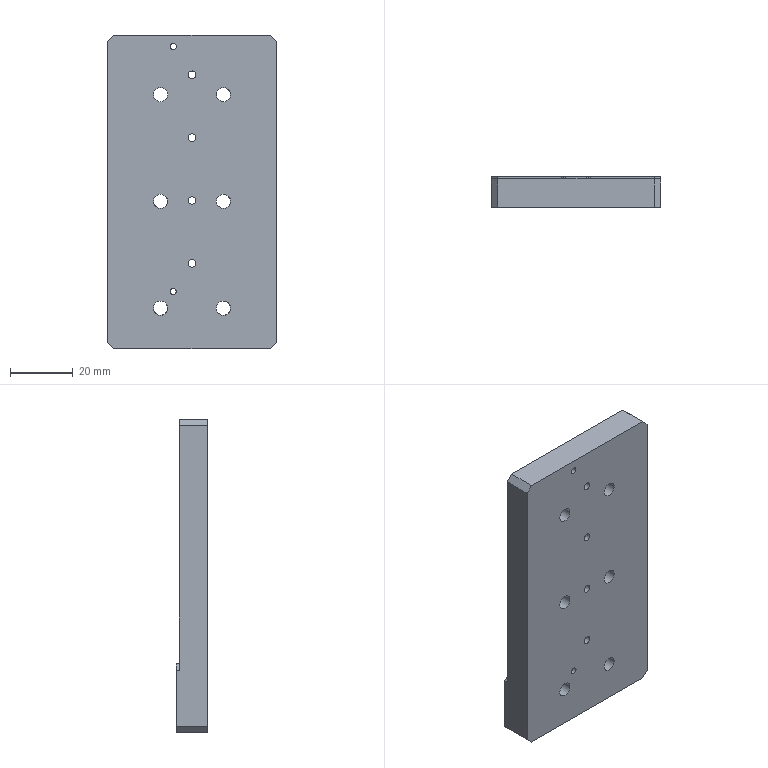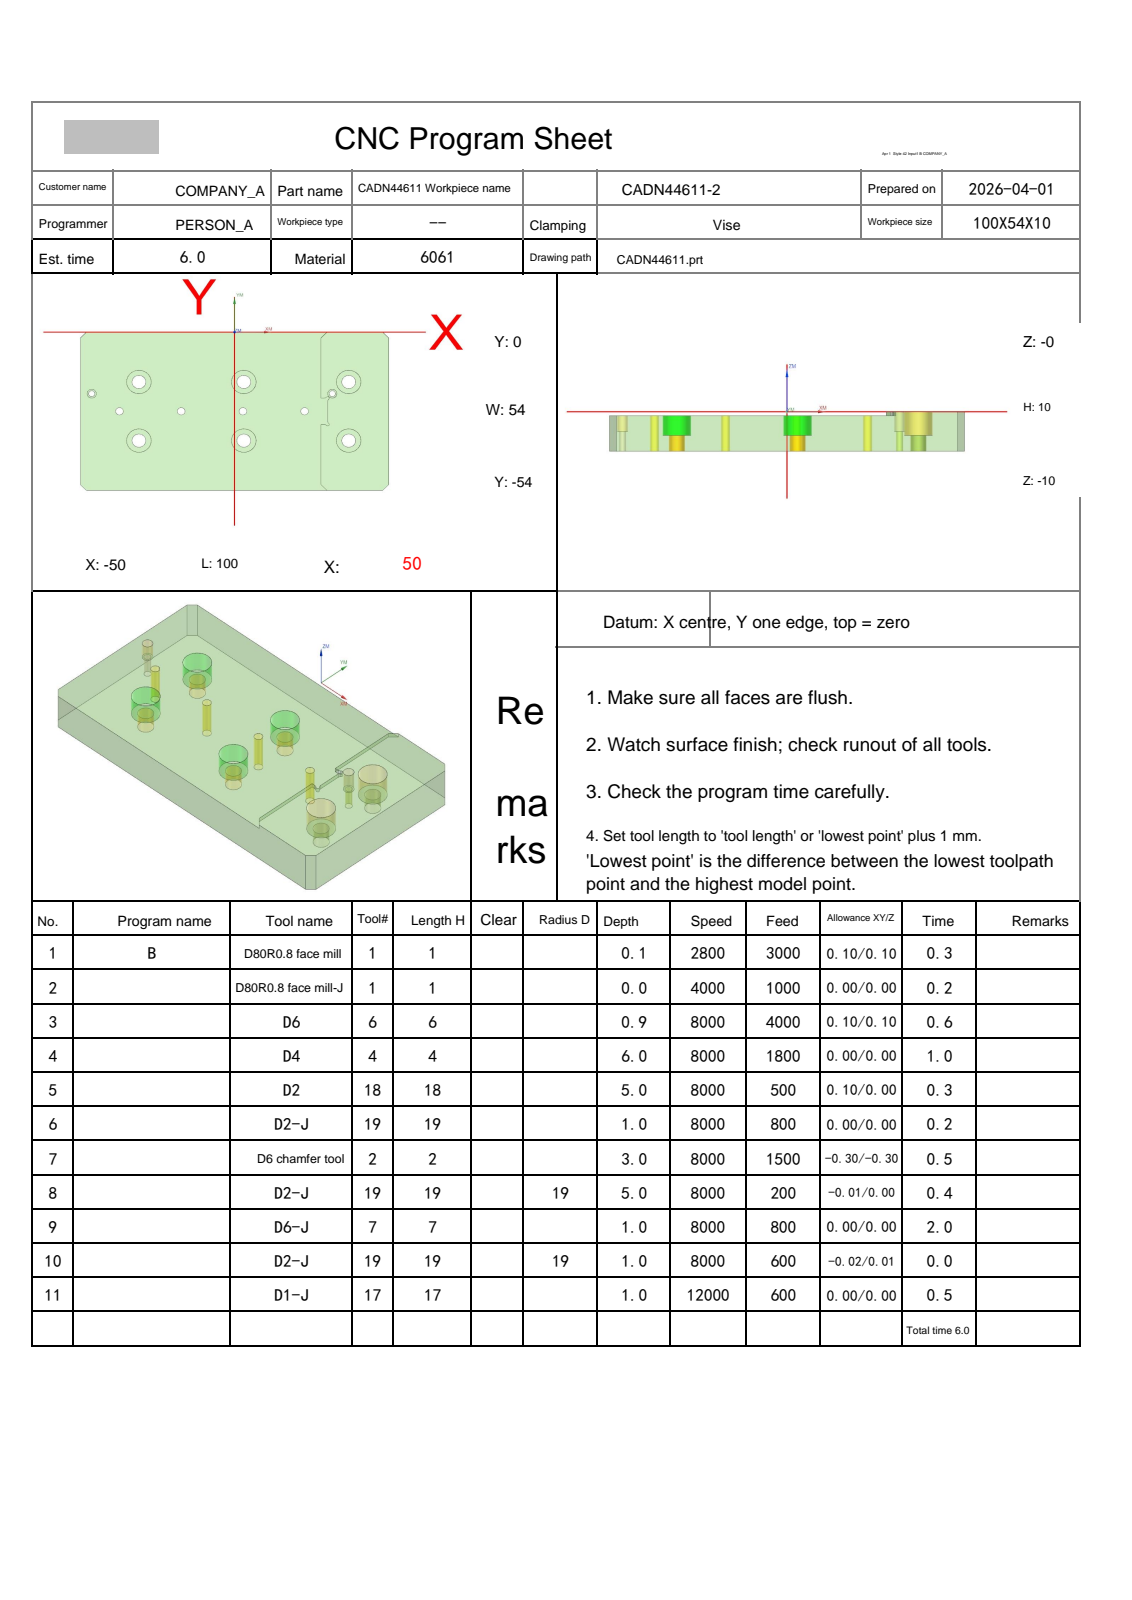NC program | NX | posted by the shop | part box 54 x 10 x 100 mm
Lines 1971 to 3760 of 3760, first 1687 of 1790 lines:
N11 T17 M06
(D1-J  D=0.96 R=0. H=17 ce=0.00 di=0.00)
G00 G90 G54 X28.679 Y-30.925 M03 S12000
G43 H17 Z20.
M08
Z.067
G01 Y-30.926 Z.052 F600.
X28.68 Y-30.93 Z.039
X28.681 Y-30.935 Z.027
X28.686 Y-30.95 Z.008
X28.695 Y-30.968 Z-.007
X28.708 Y-30.987 Z-.018
X28.725 Y-31.004 Z-.025
X28.735 Y-31.011 Z-.027
X28.747 Y-31.017 Z-.028
X28.76 Y-31.02 Z-.029
X28.775 Y-31.021
X29.082
G02 X30.186 Y-31.515 I0.0 J-1.48
G01 X30.208 Y-31.53
X30.23 Y-31.508
X30.214 Y-31.486
G02 X29.721 Y-30.383 I.987 J1.103
G01 Y-30.075
X29.713 Y-30.064 Z-.03
X29.692
X29.659 Y-30.075 Z-.031
X29.617 Y-30.096 Z-.032
X29.567 Y-30.125 Z-.033
X29.512 Y-30.161 Z-.034
X29.453 Y-30.202 Z-.036
X29.392 Y-30.247 Z-.037
X29.233 Y-30.383 Z-.042
X29.082 Y-30.533 Z-.046
X28.947 Y-30.693 Z-.051
X28.901 Y-30.754 Z-.052
X28.86 Y-30.813 Z-.054
X28.824 Y-30.868 Z-.055
X28.795 Y-30.918 Z-.056
X28.775 Y-30.96 Z-.057
X28.764 Y-30.993 Z-.058
X28.763 Y-31.014 Z-.059
X28.775 Y-31.021
X29.082
G02 X30.186 Y-31.515 I0.0 J-1.48
G01 X30.208 Y-31.53
X30.23 Y-31.508
X30.214 Y-31.486
G02 X29.721 Y-30.383 I.987 J1.103
G01 Y-30.075
X29.713 Y-30.064
X29.692
X29.659 Y-30.075 Z-.06
X29.617 Y-30.096 Z-.061
X29.567 Y-30.125 Z-.062
X29.512 Y-30.161 Z-.064
X29.453 Y-30.202 Z-.065
X29.392 Y-30.247 Z-.067
X29.233 Y-30.383 Z-.071
X29.082 Y-30.533 Z-.076
X28.947 Y-30.693 Z-.08
X28.901 Y-30.754 Z-.082
X28.86 Y-30.813 Z-.083
X28.824 Y-30.868 Z-.085
X28.795 Y-30.918 Z-.086
X28.775 Y-30.96 Z-.087
X28.764 Y-30.993 Z-.088
X28.763 Y-31.014
X28.775 Y-31.021
X29.082
G02 X30.186 Y-31.515 I0.0 J-1.48
G01 X30.208 Y-31.53
X30.23 Y-31.508
X30.214 Y-31.486
G02 X29.721 Y-30.383 I.987 J1.103
G01 Y-30.075
X29.713 Y-30.064
X29.692 Z-.089
X29.659 Y-30.075 Z-.09
X29.617 Y-30.096 Z-.091
X29.567 Y-30.125 Z-.092
X29.512 Y-30.161 Z-.093
X29.453 Y-30.202 Z-.095
X29.392 Y-30.247 Z-.096
X29.233 Y-30.383 Z-.101
X29.082 Y-30.533 Z-.105
X28.947 Y-30.693 Z-.11
X28.901 Y-30.754 Z-.111
X28.86 Y-30.813 Z-.113
X28.824 Y-30.868 Z-.114
X28.795 Y-30.918 Z-.115
X28.775 Y-30.96 Z-.116
X28.764 Y-30.993 Z-.117
X28.763 Y-31.014
X28.775 Y-31.021 Z-.118
X29.082
G02 X30.186 Y-31.515 I0.0 J-1.48
G01 X30.208 Y-31.53
X30.23 Y-31.508
X30.214 Y-31.486
G02 X29.721 Y-30.383 I.987 J1.103
G01 Y-30.075
X29.713 Y-30.064
X29.692
X29.659 Y-30.075 Z-.119
X29.617 Y-30.096 Z-.12
X29.567 Y-30.125 Z-.121
X29.512 Y-30.161 Z-.123
X29.453 Y-30.202 Z-.124
X29.392 Y-30.247 Z-.126
X29.233 Y-30.383 Z-.13
X29.082 Y-30.533 Z-.135
X28.947 Y-30.693 Z-.139
X28.901 Y-30.754 Z-.141
X28.86 Y-30.813 Z-.142
X28.824 Y-30.868 Z-.143
X28.795 Y-30.918 Z-.145
X28.775 Y-30.96 Z-.146
X28.764 Y-30.993
X28.763 Y-31.014 Z-.147
X28.775 Y-31.021
X29.082
G02 X30.186 Y-31.515 I0.0 J-1.48
G01 X30.208 Y-31.53
X30.23 Y-31.508
X30.214 Y-31.486
G02 X29.721 Y-30.383 I.987 J1.103
G01 Y-30.075
X29.713 Y-30.064
X29.692 Z-.148
X29.659 Y-30.075
X29.617 Y-30.096 Z-.149
X29.567 Y-30.125 Z-.151
X29.512 Y-30.161 Z-.152
X29.453 Y-30.202 Z-.153
X29.392 Y-30.247 Z-.155
X29.233 Y-30.383 Z-.159
X29.082 Y-30.533 Z-.164
X28.947 Y-30.693 Z-.169
X28.901 Y-30.754 Z-.17
X28.86 Y-30.813 Z-.172
X28.824 Y-30.868 Z-.173
X28.795 Y-30.918 Z-.174
X28.775 Y-30.96 Z-.175
X28.764 Y-30.993 Z-.176
X28.763 Y-31.014
X28.775 Y-31.021
X29.082
G02 X30.186 Y-31.515 I0.0 J-1.48
G01 X30.208 Y-31.53
X30.23 Y-31.508
X30.214 Y-31.486
G02 X29.721 Y-30.383 I.987 J1.103
G01 Y-30.075
X29.713 Y-30.064 Z-.177
X29.692
X29.659 Y-30.075 Z-.178
X29.617 Y-30.096 Z-.179
X29.567 Y-30.125 Z-.18
X29.512 Y-30.161 Z-.181
X29.453 Y-30.202 Z-.183
X29.392 Y-30.247 Z-.184
X29.233 Y-30.383 Z-.189
X29.082 Y-30.533 Z-.193
X28.947 Y-30.693 Z-.198
X28.901 Y-30.754 Z-.199
X28.86 Y-30.813 Z-.201
X28.824 Y-30.868 Z-.202
X28.795 Y-30.918 Z-.204
X28.775 Y-30.96
X28.764 Y-30.993 Z-.205
X28.763 Y-31.014 Z-.206
X28.775 Y-31.021
X29.082
G02 X30.186 Y-31.515 I0.0 J-1.48
G01 X30.208 Y-31.53
X30.23 Y-31.508
X30.214 Y-31.486
G02 X29.721 Y-30.383 I.987 J1.103
G01 Y-30.075
X29.713 Y-30.064
X29.692 Z-.207
X29.659 Y-30.075
X29.617 Y-30.096 Z-.208
X29.567 Y-30.125 Z-.209
X29.512 Y-30.161 Z-.211
X29.453 Y-30.202 Z-.212
X29.392 Y-30.247 Z-.214
X29.233 Y-30.383 Z-.218
X29.082 Y-30.533 Z-.223
X28.947 Y-30.693 Z-.227
X28.901 Y-30.754 Z-.229
X28.86 Y-30.813 Z-.23
X28.824 Y-30.868 Z-.232
X28.795 Y-30.918 Z-.233
X28.775 Y-30.96 Z-.234
X28.764 Y-30.993 Z-.235
X28.763 Y-31.014
X28.775 Y-31.021
X29.082
G02 X30.186 Y-31.515 I0.0 J-1.48
G01 X30.208 Y-31.53
X30.23 Y-31.508
X30.214 Y-31.486
G02 X29.721 Y-30.383 I.987 J1.103
G01 Y-30.075
X29.713 Y-30.064
X29.692 Z-.236
X29.659 Y-30.075 Z-.237
X29.617 Y-30.096 Z-.238
X29.567 Y-30.125 Z-.239
X29.512 Y-30.161 Z-.24
X29.453 Y-30.202 Z-.242
X29.392 Y-30.247 Z-.243
X29.233 Y-30.383 Z-.248
X29.082 Y-30.533 Z-.252
X28.947 Y-30.693 Z-.257
X28.901 Y-30.754 Z-.258
X28.86 Y-30.813 Z-.26
X28.824 Y-30.868 Z-.261
X28.795 Y-30.918 Z-.262
X28.775 Y-30.96 Z-.263
X28.764 Y-30.993 Z-.264
X28.763 Y-31.014 Z-.265
X28.775 Y-31.021
X29.082
G02 X30.186 Y-31.515 I0.0 J-1.48
G01 X30.208 Y-31.53
X30.23 Y-31.508
X30.214 Y-31.486
G02 X29.721 Y-30.383 I.987 J1.103
G01 Y-30.075
X29.713 Y-30.064
X29.692
X29.659 Y-30.075 Z-.266
X29.617 Y-30.096 Z-.267
X29.567 Y-30.125 Z-.268
X29.512 Y-30.161 Z-.27
X29.453 Y-30.202 Z-.271
X29.392 Y-30.247 Z-.273
X29.233 Y-30.383 Z-.277
X29.082 Y-30.533 Z-.282
X28.947 Y-30.693 Z-.286
X28.901 Y-30.754 Z-.288
X28.86 Y-30.813 Z-.289
X28.824 Y-30.868 Z-.291
X28.795 Y-30.918 Z-.292
X28.775 Y-30.96 Z-.293
X28.764 Y-30.993
X28.763 Y-31.014 Z-.294
X28.775 Y-31.021
X29.082
G02 X30.186 Y-31.515 I0.0 J-1.48
G01 X30.208 Y-31.53
X30.23 Y-31.508
X30.214 Y-31.486
G02 X29.721 Y-30.383 I.987 J1.103
G01 Y-30.075
X29.713 Y-30.064
X29.692 Z-.295
X29.659 Y-30.075 Z-.296
X29.617 Y-30.096
X29.567 Y-30.125 Z-.298
X29.512 Y-30.161 Z-.299
X29.453 Y-30.202 Z-.301
X29.392 Y-30.247 Z-.302
X29.233 Y-30.383 Z-.307
X29.082 Y-30.533 Z-.311
X28.947 Y-30.693 Z-.316
X28.901 Y-30.754 Z-.317
X28.86 Y-30.813 Z-.319
X28.824 Y-30.868 Z-.32
X28.795 Y-30.918 Z-.321
X28.775 Y-30.96 Z-.322
X28.764 Y-30.993 Z-.323
X28.763 Y-31.014
X28.775 Y-31.021 Z-.324
X29.082
G02 X30.186 Y-31.515 I0.0 J-1.48
G01 X30.208 Y-31.53
X30.23 Y-31.508
X30.214 Y-31.486
G02 X29.721 Y-30.383 I.987 J1.103
G01 Y-30.075
X29.713 Y-30.064
X29.692
X29.659 Y-30.075 Z-.325
X29.617 Y-30.096 Z-.326
X29.567 Y-30.125 Z-.327
X29.512 Y-30.161 Z-.328
X29.453 Y-30.202 Z-.33
X29.392 Y-30.247 Z-.331
X29.233 Y-30.383 Z-.336
X29.082 Y-30.533 Z-.341
X28.947 Y-30.693 Z-.345
X28.901 Y-30.754 Z-.347
X28.86 Y-30.813 Z-.348
X28.824 Y-30.868 Z-.349
X28.795 Y-30.918 Z-.351
X28.775 Y-30.96 Z-.352
X28.764 Y-30.993
X28.763 Y-31.014 Z-.353
X28.775 Y-31.021
X29.082
G02 X30.186 Y-31.515 I0.0 J-1.48
G01 X30.208 Y-31.53
X30.23 Y-31.508
X30.214 Y-31.486
G02 X29.721 Y-30.383 I.987 J1.103
G01 Y-30.075
X29.713 Y-30.064
X29.692 Z-.354
X29.659 Y-30.075
X29.617 Y-30.096 Z-.355
X29.567 Y-30.125 Z-.357
X29.512 Y-30.161 Z-.358
X29.453 Y-30.202 Z-.359
X29.392 Y-30.247 Z-.361
X29.233 Y-30.383 Z-.365
X29.082 Y-30.533 Z-.37
X28.947 Y-30.693 Z-.374
X28.901 Y-30.754 Z-.376
X28.86 Y-30.813 Z-.377
X28.824 Y-30.868 Z-.379
X28.795 Y-30.918 Z-.38
X28.775 Y-30.96 Z-.381
X28.764 Y-30.993 Z-.382
X28.763 Y-31.014
X28.775 Y-31.021
X29.082
G02 X30.186 Y-31.515 I0.0 J-1.48
G01 X30.208 Y-31.53
X30.23 Y-31.508
X30.214 Y-31.486
G02 X29.721 Y-30.383 I.987 J1.103
G01 Y-30.075
X29.713 Y-30.064 Z-.383
X29.692
X29.659 Y-30.075 Z-.384
X29.617 Y-30.096 Z-.385
X29.567 Y-30.125 Z-.386
X29.512 Y-30.161 Z-.387
X29.453 Y-30.202 Z-.389
X29.392 Y-30.247 Z-.39
X29.233 Y-30.383 Z-.395
X29.082 Y-30.533 Z-.399
X28.947 Y-30.693 Z-.404
X28.901 Y-30.754 Z-.405
X28.86 Y-30.813 Z-.407
X28.824 Y-30.868 Z-.408
X28.795 Y-30.918 Z-.409
X28.775 Y-30.96 Z-.41
X28.764 Y-30.993 Z-.411
X28.763 Y-31.014 Z-.412
X28.775 Y-31.021
X29.082
G02 X30.186 Y-31.515 I0.0 J-1.48
G01 X30.208 Y-31.53
X30.23 Y-31.508
X30.214 Y-31.486
G02 X29.721 Y-30.383 I.987 J1.103
G01 Y-30.075
X29.713 Y-30.064
X29.692
X29.659 Y-30.075 Z-.413
X29.617 Y-30.096 Z-.414
X29.567 Y-30.125 Z-.415
X29.512 Y-30.161 Z-.417
X29.453 Y-30.202 Z-.418
X29.392 Y-30.247 Z-.42
X29.233 Y-30.383 Z-.424
X29.082 Y-30.533 Z-.429
X28.947 Y-30.693 Z-.433
X28.901 Y-30.754 Z-.435
X28.86 Y-30.813 Z-.436
X28.824 Y-30.868 Z-.438
X28.795 Y-30.918 Z-.439
X28.775 Y-30.96 Z-.44
X28.764 Y-30.993 Z-.441
X28.763 Y-31.014
X28.775 Y-31.021
X29.082
G02 X30.186 Y-31.515 I0.0 J-1.48
G01 X30.208 Y-31.53
X30.23 Y-31.508
X30.214 Y-31.486
G02 X29.721 Y-30.383 I.987 J1.103
G01 Y-30.075
X29.713 Y-30.064
X29.692 Z-.442
X29.659 Y-30.075 Z-.443
X29.617 Y-30.096 Z-.444
X29.567 Y-30.125 Z-.445
X29.512 Y-30.161 Z-.446
X29.453 Y-30.202 Z-.448
X29.392 Y-30.247 Z-.449
X29.233 Y-30.383 Z-.454
X29.082 Y-30.533 Z-.458
X28.947 Y-30.693 Z-.463
X28.901 Y-30.754 Z-.464
X28.86 Y-30.813 Z-.466
X28.824 Y-30.868 Z-.467
X28.795 Y-30.918 Z-.468
X28.775 Y-30.96 Z-.469
X28.764 Y-30.993 Z-.47
X28.763 Y-31.014
X28.775 Y-31.021 Z-.471
X29.082
G02 X30.186 Y-31.515 I0.0 J-1.48
G01 X30.208 Y-31.53
X30.23 Y-31.508
X30.214 Y-31.486
G02 X29.721 Y-30.383 I.987 J1.103
G01 Y-30.075
X29.713 Y-30.064
X29.692
X29.659 Y-30.075 Z-.472
X29.617 Y-30.096 Z-.473
X29.567 Y-30.125 Z-.474
X29.512 Y-30.161 Z-.476
X29.453 Y-30.202 Z-.477
X29.392 Y-30.247 Z-.479
X29.233 Y-30.383 Z-.483
X29.082 Y-30.533 Z-.488
X28.947 Y-30.693 Z-.492
X28.901 Y-30.754 Z-.494
X28.86 Y-30.813 Z-.495
X28.824 Y-30.868 Z-.496
X28.795 Y-30.918 Z-.498
X28.775 Y-30.96 Z-.499
X28.764 Y-30.993
X28.763 Y-31.014 Z-.5
X28.775 Y-31.021
X29.082
G02 X30.186 Y-31.515 I0.0 J-1.48
G01 X30.208 Y-31.53
X30.23 Y-31.508
X30.214 Y-31.486
G02 X29.721 Y-30.383 I.987 J1.103
G01 Y-30.075
X29.713 Y-30.064
X29.692 Z-.501
X29.659 Y-30.075
X29.617 Y-30.096 Z-.502
X29.567 Y-30.125 Z-.504
X29.512 Y-30.161 Z-.505
X29.453 Y-30.202 Z-.506
X29.392 Y-30.247 Z-.508
X29.233 Y-30.383 Z-.512
X29.082 Y-30.533 Z-.517
X28.947 Y-30.693 Z-.521
X28.901 Y-30.754 Z-.523
X28.86 Y-30.813 Z-.525
X28.824 Y-30.868 Z-.526
X28.795 Y-30.918 Z-.527
X28.775 Y-30.96 Z-.528
X28.764 Y-30.993 Z-.529
X28.763 Y-31.014
X28.775 Y-31.021
X29.082
G02 X30.186 Y-31.515 I0.0 J-1.48
G01 X30.208 Y-31.53
X30.23 Y-31.508
X30.214 Y-31.486
G02 X29.721 Y-30.383 I.987 J1.103
G01 Y-30.075
X29.713 Y-30.064 Z-.53
X29.692
X29.659 Y-30.075 Z-.531
X29.617 Y-30.096 Z-.532
X29.567 Y-30.125 Z-.533
X29.512 Y-30.161 Z-.534
X29.453 Y-30.202 Z-.536
X29.392 Y-30.247 Z-.537
X29.233 Y-30.383 Z-.542
X29.082 Y-30.533 Z-.546
X28.947 Y-30.693 Z-.551
X28.901 Y-30.754 Z-.552
X28.86 Y-30.813 Z-.554
X28.824 Y-30.868 Z-.555
X28.795 Y-30.918 Z-.556
X28.775 Y-30.96 Z-.557
X28.764 Y-30.993 Z-.558
X28.763 Y-31.014 Z-.559
X28.775 Y-31.021
X29.082
G02 X30.186 Y-31.515 I0.0 J-1.48
G01 X30.208 Y-31.53
X30.23 Y-31.508
X30.214 Y-31.486
G02 X29.721 Y-30.383 I.987 J1.103
G01 Y-30.075
X29.713 Y-30.064
X29.692
X29.659 Y-30.075 Z-.56
X29.617 Y-30.096 Z-.561
X29.567 Y-30.125 Z-.562
X29.512 Y-30.161 Z-.564
X29.453 Y-30.202 Z-.565
X29.392 Y-30.247 Z-.567
X29.233 Y-30.383 Z-.571
X29.082 Y-30.533 Z-.576
X28.947 Y-30.693 Z-.58
X28.901 Y-30.754 Z-.582
X28.86 Y-30.813 Z-.583
X28.824 Y-30.868 Z-.585
X28.795 Y-30.918 Z-.586
X28.775 Y-30.96 Z-.587
X28.764 Y-30.993 Z-.588
X28.763 Y-31.014
X28.775 Y-31.021
X29.082
G02 X30.186 Y-31.515 I0.0 J-1.48
G01 X30.208 Y-31.53
X30.23 Y-31.508
X30.214 Y-31.486
G02 X29.721 Y-30.383 I.987 J1.103
G01 Y-30.075
X29.713 Y-30.064
X29.692 Z-.589
X29.659 Y-30.075 Z-.59
X29.617 Y-30.096 Z-.591
X29.567 Y-30.125 Z-.592
X29.512 Y-30.161 Z-.593
X29.453 Y-30.202 Z-.595
X29.392 Y-30.247 Z-.596
X29.233 Y-30.383 Z-.601
X29.082 Y-30.533 Z-.605
X28.947 Y-30.693 Z-.61
X28.901 Y-30.754 Z-.611
X28.86 Y-30.813 Z-.613
X28.824 Y-30.868 Z-.614
X28.795 Y-30.918 Z-.615
X28.775 Y-30.96 Z-.616
X28.764 Y-30.993 Z-.617
X28.763 Y-31.014
X28.775 Y-31.021 Z-.618
X29.082
G02 X30.186 Y-31.515 I0.0 J-1.48
G01 X30.208 Y-31.53
X30.23 Y-31.508
X30.214 Y-31.486
G02 X29.721 Y-30.383 I.987 J1.103
G01 Y-30.075
X29.713 Y-30.064
X29.692
X29.659 Y-30.075 Z-.619
X29.617 Y-30.096 Z-.62
X29.567 Y-30.125 Z-.621
X29.512 Y-30.161 Z-.623
X29.453 Y-30.202 Z-.624
X29.392 Y-30.247 Z-.626
X29.233 Y-30.383 Z-.63
X29.082 Y-30.533 Z-.635
X28.947 Y-30.693 Z-.639
X28.901 Y-30.754 Z-.641
X28.86 Y-30.813 Z-.642
X28.824 Y-30.868 Z-.643
X28.795 Y-30.918 Z-.645
X28.775 Y-30.96 Z-.646
X28.764 Y-30.993
X28.763 Y-31.014 Z-.647
X28.775 Y-31.021
X29.082
G02 X30.186 Y-31.515 I0.0 J-1.48
G01 X30.208 Y-31.53
X30.23 Y-31.508
X30.214 Y-31.486
G02 X29.721 Y-30.383 I.987 J1.103
G01 Y-30.075
X29.713 Y-30.064
X29.692 Z-.648
X29.659 Y-30.075
X29.617 Y-30.096 Z-.649
X29.567 Y-30.125 Z-.651
X29.512 Y-30.161 Z-.652
X29.453 Y-30.202 Z-.653
X29.392 Y-30.247 Z-.655
X29.233 Y-30.383 Z-.659
X29.082 Y-30.533 Z-.664
X28.947 Y-30.693 Z-.669
X28.901 Y-30.754 Z-.67
X28.86 Y-30.813 Z-.672
X28.824 Y-30.868 Z-.673
X28.795 Y-30.918 Z-.674
X28.775 Y-30.96 Z-.675
X28.764 Y-30.993 Z-.676
X28.763 Y-31.014
X28.775 Y-31.021
X29.082
G02 X30.186 Y-31.515 I0.0 J-1.48
G01 X30.208 Y-31.53
X30.23 Y-31.508
X30.214 Y-31.486
G02 X29.721 Y-30.383 I.987 J1.103
G01 Y-30.075
X29.713 Y-30.064 Z-.677
X29.692
X29.659 Y-30.075 Z-.678
X29.617 Y-30.096 Z-.679
X29.567 Y-30.125 Z-.68
X29.512 Y-30.161 Z-.681
X29.453 Y-30.202 Z-.683
X29.392 Y-30.247 Z-.684
X29.233 Y-30.383 Z-.689
X29.082 Y-30.533 Z-.693
X28.947 Y-30.693 Z-.698
X28.901 Y-30.754 Z-.699
X28.86 Y-30.813 Z-.701
X28.824 Y-30.868 Z-.702
X28.795 Y-30.918 Z-.704
X28.775 Y-30.96
X28.764 Y-30.993 Z-.705
X28.763 Y-31.014 Z-.706
X28.775 Y-31.021
X29.082
G02 X30.186 Y-31.515 I0.0 J-1.48
G01 X30.208 Y-31.53
X30.23 Y-31.508
X30.214 Y-31.486
G02 X29.721 Y-30.383 I.987 J1.103
G01 Y-30.075
X29.713 Y-30.064
X29.692 Z-.707
X29.659 Y-30.075
X29.617 Y-30.096 Z-.708
X29.567 Y-30.125 Z-.709
X29.512 Y-30.161 Z-.711
X29.453 Y-30.202 Z-.712
X29.392 Y-30.247 Z-.714
X29.233 Y-30.383 Z-.718
X29.082 Y-30.533 Z-.723
X28.947 Y-30.693 Z-.727
X28.901 Y-30.754 Z-.729
X28.86 Y-30.813 Z-.73
X28.824 Y-30.868 Z-.732
X28.795 Y-30.918 Z-.733
X28.775 Y-30.96 Z-.734
X28.764 Y-30.993 Z-.735
X28.763 Y-31.014
X28.775 Y-31.021
X29.082
G02 X30.186 Y-31.515 I0.0 J-1.48
G01 X30.208 Y-31.53
X30.23 Y-31.508
X30.214 Y-31.486
G02 X29.721 Y-30.383 I.987 J1.103
G01 Y-30.075
X29.713 Y-30.064
X29.692 Z-.736
X29.659 Y-30.075 Z-.737
X29.617 Y-30.096 Z-.738
X29.567 Y-30.125 Z-.739
X29.512 Y-30.161 Z-.74
X29.453 Y-30.202 Z-.742
X29.392 Y-30.247 Z-.743
X29.233 Y-30.383 Z-.748
X29.082 Y-30.533 Z-.752
X28.947 Y-30.693 Z-.757
X28.901 Y-30.754 Z-.758
X28.86 Y-30.813 Z-.76
X28.824 Y-30.868 Z-.761
X28.795 Y-30.918 Z-.762
X28.775 Y-30.96 Z-.763
X28.764 Y-30.993 Z-.764
X28.763 Y-31.014 Z-.765
X28.775 Y-31.021
X29.082
G02 X30.186 Y-31.515 I0.0 J-1.48
G01 X30.208 Y-31.53
X30.23 Y-31.508
X30.214 Y-31.486
G02 X29.721 Y-30.383 I.987 J1.103
G01 Y-30.075
X29.713 Y-30.064
X29.692
X29.659 Y-30.075 Z-.766
X29.617 Y-30.096 Z-.767
X29.567 Y-30.125 Z-.768
X29.512 Y-30.161 Z-.77
X29.453 Y-30.202 Z-.771
X29.392 Y-30.247 Z-.773
X29.233 Y-30.383 Z-.777
X29.082 Y-30.533 Z-.782
X28.947 Y-30.693 Z-.786
X28.901 Y-30.754 Z-.788
X28.86 Y-30.813 Z-.789
X28.824 Y-30.868 Z-.791
X28.795 Y-30.918 Z-.792
X28.775 Y-30.96 Z-.793
X28.764 Y-30.993
X28.763 Y-31.014 Z-.794
X28.775 Y-31.021
X29.082
G02 X30.186 Y-31.515 I0.0 J-1.48
G01 X30.208 Y-31.53
X30.23 Y-31.508
X30.214 Y-31.486
G02 X29.721 Y-30.383 I.987 J1.103
G01 Y-30.075
X29.713 Y-30.064
X29.692 Z-.795
X29.659 Y-30.075 Z-.796
X29.617 Y-30.096
X29.567 Y-30.125 Z-.798
X29.512 Y-30.161 Z-.799
X29.453 Y-30.202 Z-.801
X29.392 Y-30.247 Z-.802
X29.233 Y-30.383 Z-.807
X29.082 Y-30.533 Z-.811
X28.947 Y-30.693 Z-.816
X28.901 Y-30.754 Z-.817
X28.86 Y-30.813 Z-.819
X28.824 Y-30.868 Z-.82
X28.795 Y-30.918 Z-.821
X28.775 Y-30.96 Z-.822
X28.764 Y-30.993 Z-.823
X28.763 Y-31.014
X28.775 Y-31.021 Z-.824
X29.082
G02 X30.186 Y-31.515 I0.0 J-1.48
G01 X30.208 Y-31.53
X30.23 Y-31.508
X30.214 Y-31.486
G02 X29.721 Y-30.383 I.987 J1.103
G01 Y-30.075
X29.713 Y-30.064
X29.692
X29.659 Y-30.075 Z-.825
X29.617 Y-30.096 Z-.826
X29.567 Y-30.125 Z-.827
X29.512 Y-30.161 Z-.828
X29.453 Y-30.202 Z-.83
X29.392 Y-30.247 Z-.831
X29.233 Y-30.383 Z-.836
X29.082 Y-30.533 Z-.841
X28.947 Y-30.693 Z-.845
X28.901 Y-30.754 Z-.847
X28.86 Y-30.813 Z-.848
X28.824 Y-30.868 Z-.849
X28.795 Y-30.918 Z-.851
X28.775 Y-30.96 Z-.852
X28.764 Y-30.993
X28.763 Y-31.014 Z-.853
X28.775 Y-31.021
X29.082
G02 X30.186 Y-31.515 I0.0 J-1.48
G01 X30.208 Y-31.53
X30.23 Y-31.508
X30.214 Y-31.486
G02 X29.721 Y-30.383 I.987 J1.103
G01 Y-30.075
X29.713 Y-30.064
X29.692 Z-.854
X29.659 Y-30.075
X29.617 Y-30.096 Z-.855
X29.567 Y-30.125 Z-.857
X29.512 Y-30.161 Z-.858
X29.453 Y-30.202 Z-.859
X29.392 Y-30.247 Z-.861
X29.233 Y-30.383 Z-.865
X29.082 Y-30.533 Z-.87
X28.947 Y-30.693 Z-.874
X28.901 Y-30.754 Z-.876
X28.86 Y-30.813 Z-.877
X28.824 Y-30.868 Z-.879
X28.795 Y-30.918 Z-.88
X28.775 Y-30.96 Z-.881
X28.764 Y-30.993 Z-.882
X28.763 Y-31.014
X28.775 Y-31.021
X29.082
G02 X30.186 Y-31.515 I0.0 J-1.48
G01 X30.208 Y-31.53
X30.23 Y-31.508
X30.214 Y-31.486
G02 X29.721 Y-30.383 I.987 J1.103
G01 Y-30.075
X29.713 Y-30.064 Z-.883
X29.692
X29.659 Y-30.075 Z-.884
X29.617 Y-30.096 Z-.885
X29.567 Y-30.125 Z-.886
X29.512 Y-30.161 Z-.887
X29.453 Y-30.202 Z-.889
X29.392 Y-30.247 Z-.89
X29.233 Y-30.383 Z-.895
X29.082 Y-30.533 Z-.899
X28.947 Y-30.693 Z-.904
X28.901 Y-30.754 Z-.905
X28.86 Y-30.813 Z-.907
X28.824 Y-30.868 Z-.908
X28.795 Y-30.918 Z-.909
X28.775 Y-30.96 Z-.91
X28.764 Y-30.993 Z-.911
X28.763 Y-31.014 Z-.912
X28.775 Y-31.021
X29.082
G02 X30.186 Y-31.515 I0.0 J-1.48
G01 X30.208 Y-31.53
X30.23 Y-31.508
X30.214 Y-31.486
G02 X29.721 Y-30.383 I.987 J1.103
G01 Y-30.075
X29.713 Y-30.064
X29.692
X29.659 Y-30.075 Z-.913
X29.617 Y-30.096 Z-.914
X29.567 Y-30.125 Z-.915
X29.512 Y-30.161 Z-.917
X29.453 Y-30.202 Z-.918
X29.392 Y-30.247 Z-.92
X29.233 Y-30.383 Z-.924
X29.082 Y-30.533 Z-.929
X28.947 Y-30.693 Z-.933
X28.901 Y-30.754 Z-.935
X28.86 Y-30.813 Z-.936
X28.824 Y-30.868 Z-.938
X28.795 Y-30.918 Z-.939
X28.775 Y-30.96 Z-.94
X28.764 Y-30.993 Z-.941
X28.763 Y-31.014
X28.775 Y-31.021
X29.082
G02 X30.186 Y-31.515 I0.0 J-1.48
G01 X30.208 Y-31.53
X30.23 Y-31.508
X30.214 Y-31.486
G02 X29.721 Y-30.383 I.987 J1.103
G01 Y-30.075
X29.713 Y-30.064
X29.692 Z-.942
X29.659 Y-30.075 Z-.943
X29.617 Y-30.096 Z-.944
X29.567 Y-30.125 Z-.945
X29.512 Y-30.161 Z-.946
X29.453 Y-30.202 Z-.948
X29.392 Y-30.247 Z-.949
X29.233 Y-30.383 Z-.954
X29.082 Y-30.533 Z-.958
X28.947 Y-30.693 Z-.963
X28.901 Y-30.754 Z-.964
X28.86 Y-30.813 Z-.966
X28.824 Y-30.868 Z-.967
X28.795 Y-30.918 Z-.968
X28.775 Y-30.96 Z-.969
X28.764 Y-30.993 Z-.97
X28.763 Y-31.014
X28.775 Y-31.021 Z-.971
X29.082
G02 X30.186 Y-31.515 I0.0 J-1.48
G01 X30.208 Y-31.53
X30.23 Y-31.508
X30.214 Y-31.486
G02 X29.721 Y-30.383 I.987 J1.103
G01 Y-30.075
X29.713 Y-30.064
X29.692
X29.659 Y-30.075 Z-.972
X29.617 Y-30.096 Z-.973
X29.567 Y-30.125 Z-.974
X29.512 Y-30.161 Z-.976
X29.453 Y-30.202 Z-.977
X29.392 Y-30.247 Z-.979
X29.233 Y-30.383 Z-.983
X29.082 Y-30.533 Z-.988
X28.947 Y-30.693 Z-.992
X28.901 Y-30.754 Z-.994
X28.86 Y-30.813 Z-.995
X28.824 Y-30.868 Z-.996
X28.795 Y-30.918 Z-.998
X28.775 Y-30.96 Z-.999
X28.764 Y-30.993
X28.763 Y-31.014 Z-1.
X28.775 Y-31.021
X29.082
G02 X30.186 Y-31.515 I0.0 J-1.48
G01 X30.208 Y-31.53
X30.23 Y-31.508
X30.214 Y-31.486
G02 X29.721 Y-30.383 I.987 J1.103
G01 Y-30.075
X29.719 Y-30.061
X29.716 Y-30.047 Z-.999
X29.711 Y-30.036 Z-.997
X29.696 Y-30.016 Z-.992
X29.677 Y-30.001 Z-.984
X29.658 Y-29.991 Z-.971
X29.641 Y-29.984 Z-.954
X29.635 Y-29.982 Z-.943
X29.629 Y-29.98 Z-.932
X29.626 Y-29.979 Z-.919
X29.625 Z-.904
G00 Z3.
Y-24.023
Z.067
G01 X29.626 Z.052
X29.629 Y-24.022 Z.039
X29.635 Y-24.021 Z.027
X29.649 Y-24.015 Z.008
X29.668 Y-24.007 Z-.007
X29.687 Y-23.994 Z-.018
X29.704 Y-23.977 Z-.025
X29.711 Y-23.967 Z-.027
X29.716 Y-23.955 Z-.028
X29.719 Y-23.942 Z-.029
X29.721 Y-23.927
Y-23.619
G02 X30.214 Y-22.516 I1.48 J0.0
G01 X30.23 Y-22.494
X30.208 Y-22.472
X30.186 Y-22.488
G02 X29.083 Y-22.981 I-1.103 J.987
G01 X28.775
X28.763 Y-22.989 Z-.03
X28.764 Y-23.01
X28.775 Y-23.042 Z-.031
X28.795 Y-23.085 Z-.032
X28.824 Y-23.134 Z-.033
X28.86 Y-23.19 Z-.034
X28.901 Y-23.249 Z-.036
X28.947 Y-23.309 Z-.037
X29.082 Y-23.469 Z-.042
X29.233 Y-23.619 Z-.046
X29.392 Y-23.755 Z-.051
X29.453 Y-23.801 Z-.052
X29.512 Y-23.842 Z-.054
X29.567 Y-23.877 Z-.055
X29.617 Y-23.906 Z-.056
X29.659 Y-23.927 Z-.057
X29.692 Y-23.938 Z-.058
X29.713 Y-23.939 Z-.059
X29.721 Y-23.927
Y-23.619
G02 X30.214 Y-22.516 I1.48 J0.0
G01 X30.23 Y-22.494
X30.208 Y-22.472
X30.186 Y-22.488
G02 X29.083 Y-22.981 I-1.103 J.987
G01 X28.775
X28.763 Y-22.989
X28.764 Y-23.01
X28.775 Y-23.042 Z-.06
X28.795 Y-23.085 Z-.061
X28.824 Y-23.134 Z-.062
X28.86 Y-23.19 Z-.064
X28.901 Y-23.249 Z-.065
X28.947 Y-23.309 Z-.067
X29.082 Y-23.469 Z-.071
X29.233 Y-23.619 Z-.076
X29.392 Y-23.755 Z-.08
X29.453 Y-23.801 Z-.082
X29.512 Y-23.842 Z-.083
X29.567 Y-23.877 Z-.085
X29.617 Y-23.906 Z-.086
X29.659 Y-23.927 Z-.087
X29.692 Y-23.938 Z-.088
X29.713 Y-23.939
X29.721 Y-23.927
Y-23.619
G02 X30.214 Y-22.516 I1.48 J0.0
G01 X30.23 Y-22.494
X30.208 Y-22.472
X30.186 Y-22.488
G02 X29.083 Y-22.981 I-1.103 J.987
G01 X28.775
X28.763 Y-22.989
X28.764 Y-23.01 Z-.089
X28.775 Y-23.042 Z-.09
X28.795 Y-23.085 Z-.091
X28.824 Y-23.134 Z-.092
X28.86 Y-23.19 Z-.093
X28.901 Y-23.249 Z-.095
X28.947 Y-23.309 Z-.096
X29.082 Y-23.469 Z-.101
X29.233 Y-23.619 Z-.105
X29.392 Y-23.755 Z-.11
X29.453 Y-23.801 Z-.111
X29.512 Y-23.842 Z-.113
X29.567 Y-23.877 Z-.114
X29.617 Y-23.906 Z-.115
X29.659 Y-23.927 Z-.116
X29.692 Y-23.938 Z-.117
X29.713 Y-23.939
X29.721 Y-23.927 Z-.118
Y-23.619
G02 X30.214 Y-22.516 I1.48 J0.0
G01 X30.23 Y-22.494
X30.208 Y-22.472
X30.186 Y-22.488
G02 X29.083 Y-22.981 I-1.103 J.987
G01 X28.775
X28.763 Y-22.989
X28.764 Y-23.01
X28.775 Y-23.042 Z-.119
X28.795 Y-23.085 Z-.12
X28.824 Y-23.134 Z-.121
X28.86 Y-23.19 Z-.123
X28.901 Y-23.249 Z-.124
X28.947 Y-23.309 Z-.126
X29.082 Y-23.469 Z-.13
X29.233 Y-23.619 Z-.135
X29.392 Y-23.755 Z-.139
X29.453 Y-23.801 Z-.141
X29.512 Y-23.842 Z-.142
X29.567 Y-23.877 Z-.143
X29.617 Y-23.906 Z-.145
X29.659 Y-23.927 Z-.146
X29.692 Y-23.938
X29.713 Y-23.939 Z-.147
X29.721 Y-23.927
Y-23.619
G02 X30.214 Y-22.516 I1.48 J0.0
G01 X30.23 Y-22.494
X30.208 Y-22.472
X30.186 Y-22.488
G02 X29.083 Y-22.981 I-1.103 J.987
G01 X28.775
X28.763 Y-22.989
X28.764 Y-23.01 Z-.148
X28.775 Y-23.042
X28.795 Y-23.085 Z-.149
X28.824 Y-23.134 Z-.151
X28.86 Y-23.19 Z-.152
X28.901 Y-23.249 Z-.153
X28.947 Y-23.309 Z-.155
X29.082 Y-23.469 Z-.159
X29.233 Y-23.619 Z-.164
X29.392 Y-23.755 Z-.169
X29.453 Y-23.801 Z-.17
X29.512 Y-23.842 Z-.172
X29.567 Y-23.877 Z-.173
X29.617 Y-23.906 Z-.174
X29.659 Y-23.927 Z-.175
X29.692 Y-23.938 Z-.176
X29.713 Y-23.939
X29.721 Y-23.927
Y-23.619
G02 X30.214 Y-22.516 I1.48 J0.0
G01 X30.23 Y-22.494
X30.208 Y-22.472
X30.186 Y-22.488
G02 X29.083 Y-22.981 I-1.103 J.987
G01 X28.775
X28.763 Y-22.989 Z-.177
X28.764 Y-23.01
X28.775 Y-23.042 Z-.178
X28.795 Y-23.085 Z-.179
X28.824 Y-23.134 Z-.18
X28.86 Y-23.19 Z-.181
X28.901 Y-23.249 Z-.183
X28.947 Y-23.309 Z-.184
X29.082 Y-23.469 Z-.189
X29.233 Y-23.619 Z-.193
X29.392 Y-23.755 Z-.198
X29.453 Y-23.801 Z-.199
X29.512 Y-23.842 Z-.201
X29.567 Y-23.877 Z-.202
X29.617 Y-23.906 Z-.204
X29.659 Y-23.927
X29.692 Y-23.938 Z-.205
X29.713 Y-23.939 Z-.206
X29.721 Y-23.927
Y-23.619
G02 X30.214 Y-22.516 I1.48 J0.0
G01 X30.23 Y-22.494
X30.208 Y-22.472
X30.186 Y-22.488
G02 X29.083 Y-22.981 I-1.103 J.987
G01 X28.775
X28.763 Y-22.989
X28.764 Y-23.01 Z-.207
X28.775 Y-23.042
X28.795 Y-23.085 Z-.208
X28.824 Y-23.134 Z-.209
X28.86 Y-23.19 Z-.211
X28.901 Y-23.249 Z-.212
X28.947 Y-23.309 Z-.214
X29.082 Y-23.469 Z-.218
X29.233 Y-23.619 Z-.223
X29.392 Y-23.755 Z-.227
X29.453 Y-23.801 Z-.229
X29.512 Y-23.842 Z-.23
X29.567 Y-23.877 Z-.232
X29.617 Y-23.906 Z-.233
X29.659 Y-23.927 Z-.234
X29.692 Y-23.938 Z-.235
X29.713 Y-23.939
X29.721 Y-23.927
Y-23.619
G02 X30.214 Y-22.516 I1.48 J0.0
G01 X30.23 Y-22.494
X30.208 Y-22.472
X30.186 Y-22.488
G02 X29.083 Y-22.981 I-1.103 J.987
G01 X28.775
X28.763 Y-22.989
X28.764 Y-23.01 Z-.236
X28.775 Y-23.042 Z-.237
X28.795 Y-23.085 Z-.238
X28.824 Y-23.134 Z-.239
X28.86 Y-23.19 Z-.24
X28.901 Y-23.249 Z-.242
X28.947 Y-23.309 Z-.243
X29.082 Y-23.469 Z-.248
X29.233 Y-23.619 Z-.252
X29.392 Y-23.755 Z-.257
X29.453 Y-23.801 Z-.258
X29.512 Y-23.842 Z-.26
X29.567 Y-23.877 Z-.261
X29.617 Y-23.906 Z-.262
X29.659 Y-23.927 Z-.263
X29.692 Y-23.938 Z-.264
X29.713 Y-23.939 Z-.265
X29.721 Y-23.927
Y-23.619
G02 X30.214 Y-22.516 I1.48 J0.0
G01 X30.23 Y-22.494
X30.208 Y-22.472
X30.186 Y-22.488
G02 X29.083 Y-22.981 I-1.103 J.987
G01 X28.775
X28.763 Y-22.989
X28.764 Y-23.01
X28.775 Y-23.042 Z-.266
X28.795 Y-23.085 Z-.267
X28.824 Y-23.134 Z-.268
X28.86 Y-23.19 Z-.27
X28.901 Y-23.249 Z-.271
X28.947 Y-23.309 Z-.273
X29.082 Y-23.469 Z-.277
X29.233 Y-23.619 Z-.282
X29.392 Y-23.755 Z-.286
X29.453 Y-23.801 Z-.288
X29.512 Y-23.842 Z-.289
X29.567 Y-23.877 Z-.291
X29.617 Y-23.906 Z-.292
X29.659 Y-23.927 Z-.293
X29.692 Y-23.938
X29.713 Y-23.939 Z-.294
X29.721 Y-23.927
Y-23.619
G02 X30.214 Y-22.516 I1.48 J0.0
G01 X30.23 Y-22.494
X30.208 Y-22.472
X30.186 Y-22.488
G02 X29.083 Y-22.981 I-1.103 J.987
G01 X28.775
X28.763 Y-22.989
X28.764 Y-23.01 Z-.295
X28.775 Y-23.042 Z-.296
X28.795 Y-23.085
X28.824 Y-23.134 Z-.298
X28.86 Y-23.19 Z-.299
X28.901 Y-23.249 Z-.301
X28.947 Y-23.309 Z-.302
X29.082 Y-23.469 Z-.307
X29.233 Y-23.619 Z-.311
X29.392 Y-23.755 Z-.316
X29.453 Y-23.801 Z-.317
X29.512 Y-23.842 Z-.319
X29.567 Y-23.877 Z-.32
X29.617 Y-23.906 Z-.321
X29.659 Y-23.927 Z-.322
X29.692 Y-23.938 Z-.323
X29.713 Y-23.939
X29.721 Y-23.927 Z-.324
Y-23.619
G02 X30.214 Y-22.516 I1.48 J0.0
G01 X30.23 Y-22.494
X30.208 Y-22.472
X30.186 Y-22.488
G02 X29.083 Y-22.981 I-1.103 J.987
G01 X28.775
X28.763 Y-22.989
X28.764 Y-23.01
X28.775 Y-23.042 Z-.325
X28.795 Y-23.085 Z-.326
X28.824 Y-23.134 Z-.327
X28.86 Y-23.19 Z-.328
X28.901 Y-23.249 Z-.33
X28.947 Y-23.309 Z-.331
X29.082 Y-23.469 Z-.336
X29.233 Y-23.619 Z-.341
X29.392 Y-23.755 Z-.345
X29.453 Y-23.801 Z-.347
X29.512 Y-23.842 Z-.348
X29.567 Y-23.877 Z-.349
X29.617 Y-23.906 Z-.351
X29.659 Y-23.927 Z-.352
X29.692 Y-23.938
X29.713 Y-23.939 Z-.353
X29.721 Y-23.927
Y-23.619
G02 X30.214 Y-22.516 I1.48 J0.0
G01 X30.23 Y-22.494
X30.208 Y-22.472
X30.186 Y-22.488
G02 X29.083 Y-22.981 I-1.103 J.987
G01 X28.775
X28.763 Y-22.989
X28.764 Y-23.01 Z-.354
X28.775 Y-23.042
X28.795 Y-23.085 Z-.355
X28.824 Y-23.134 Z-.357
X28.86 Y-23.19 Z-.358
X28.901 Y-23.249 Z-.359
X28.947 Y-23.309 Z-.361
X29.082 Y-23.469 Z-.365
X29.233 Y-23.619 Z-.37
X29.392 Y-23.755 Z-.374
X29.453 Y-23.801 Z-.376
X29.512 Y-23.842 Z-.377
X29.567 Y-23.877 Z-.379
X29.617 Y-23.906 Z-.38
X29.659 Y-23.927 Z-.381
X29.692 Y-23.938 Z-.382
X29.713 Y-23.939
X29.721 Y-23.927
Y-23.619
G02 X30.214 Y-22.516 I1.48 J0.0
G01 X30.23 Y-22.494
X30.208 Y-22.472
X30.186 Y-22.488
G02 X29.083 Y-22.981 I-1.103 J.987
G01 X28.775
X28.763 Y-22.989 Z-.383
X28.764 Y-23.01
X28.775 Y-23.042 Z-.384
X28.795 Y-23.085 Z-.385
X28.824 Y-23.134 Z-.386
X28.86 Y-23.19 Z-.387
X28.901 Y-23.249 Z-.389
X28.947 Y-23.309 Z-.39
X29.082 Y-23.469 Z-.395
X29.233 Y-23.619 Z-.399
X29.392 Y-23.755 Z-.404
X29.453 Y-23.801 Z-.405
X29.512 Y-23.842 Z-.407
X29.567 Y-23.877 Z-.408
X29.617 Y-23.906 Z-.409
X29.659 Y-23.927 Z-.41
X29.692 Y-23.938 Z-.411
X29.713 Y-23.939 Z-.412
X29.721 Y-23.927
Y-23.619
G02 X30.214 Y-22.516 I1.48 J0.0
G01 X30.23 Y-22.494
X30.208 Y-22.472
X30.186 Y-22.488
G02 X29.083 Y-22.981 I-1.103 J.987
G01 X28.775
X28.763 Y-22.989
X28.764 Y-23.01
X28.775 Y-23.042 Z-.413
X28.795 Y-23.085 Z-.414
X28.824 Y-23.134 Z-.415
X28.86 Y-23.19 Z-.417
X28.901 Y-23.249 Z-.418
X28.947 Y-23.309 Z-.42
X29.082 Y-23.469 Z-.424
X29.233 Y-23.619 Z-.429
X29.392 Y-23.755 Z-.433
X29.453 Y-23.801 Z-.435
X29.512 Y-23.842 Z-.436
X29.567 Y-23.877 Z-.438
X29.617 Y-23.906 Z-.439
X29.659 Y-23.927 Z-.44
X29.692 Y-23.938 Z-.441
X29.713 Y-23.939
X29.721 Y-23.927
Y-23.619
G02 X30.214 Y-22.516 I1.48 J0.0
G01 X30.23 Y-22.494
X30.208 Y-22.472
X30.186 Y-22.488
G02 X29.083 Y-22.981 I-1.103 J.987
G01 X28.775
X28.763 Y-22.989
X28.764 Y-23.01 Z-.442
X28.775 Y-23.042 Z-.443
X28.795 Y-23.085 Z-.444
X28.824 Y-23.134 Z-.445
X28.86 Y-23.19 Z-.446
X28.901 Y-23.249 Z-.448
X28.947 Y-23.309 Z-.449
X29.082 Y-23.469 Z-.454
X29.233 Y-23.619 Z-.458
X29.392 Y-23.755 Z-.463
X29.453 Y-23.801 Z-.464
X29.512 Y-23.842 Z-.466
X29.567 Y-23.877 Z-.467
X29.617 Y-23.906 Z-.468
X29.659 Y-23.927 Z-.469
X29.692 Y-23.938 Z-.47
X29.713 Y-23.939
X29.721 Y-23.927 Z-.471
Y-23.619
G02 X30.214 Y-22.516 I1.48 J0.0
G01 X30.23 Y-22.494
X30.208 Y-22.472
X30.186 Y-22.488
G02 X29.083 Y-22.981 I-1.103 J.987
G01 X28.775
X28.763 Y-22.989
X28.764 Y-23.01
X28.775 Y-23.042 Z-.472
X28.795 Y-23.085 Z-.473
X28.824 Y-23.134 Z-.474
X28.86 Y-23.19 Z-.476
X28.901 Y-23.249 Z-.477
X28.947 Y-23.309 Z-.479
X29.082 Y-23.469 Z-.483
X29.233 Y-23.619 Z-.488
X29.392 Y-23.755 Z-.492
X29.453 Y-23.801 Z-.494
X29.512 Y-23.842 Z-.495
X29.567 Y-23.877 Z-.496
X29.617 Y-23.906 Z-.498
X29.659 Y-23.927 Z-.499
X29.692 Y-23.938
X29.713 Y-23.939 Z-.5
X29.721 Y-23.927
Y-23.619
G02 X30.214 Y-22.516 I1.48 J0.0
G01 X30.23 Y-22.494
X30.208 Y-22.472
X30.186 Y-22.488
G02 X29.083 Y-22.981 I-1.103 J.987
G01 X28.775
X28.763 Y-22.989
X28.764 Y-23.01 Z-.501
X28.775 Y-23.042
X28.795 Y-23.085 Z-.502
X28.824 Y-23.134 Z-.504
X28.86 Y-23.19 Z-.505
X28.901 Y-23.249 Z-.506
X28.947 Y-23.309 Z-.508
X29.082 Y-23.469 Z-.512
X29.233 Y-23.619 Z-.517
X29.392 Y-23.755 Z-.521
X29.453 Y-23.801 Z-.523
X29.512 Y-23.842 Z-.525
X29.567 Y-23.877 Z-.526
X29.617 Y-23.906 Z-.527
X29.659 Y-23.927 Z-.528
X29.692 Y-23.938 Z-.529
X29.713 Y-23.939
X29.721 Y-23.927
Y-23.619
G02 X30.214 Y-22.516 I1.48 J0.0
G01 X30.23 Y-22.494
X30.208 Y-22.472
X30.186 Y-22.488
G02 X29.083 Y-22.981 I-1.103 J.987
G01 X28.775
X28.763 Y-22.989 Z-.53
X28.764 Y-23.01
X28.775 Y-23.042 Z-.531
X28.795 Y-23.085 Z-.532
X28.824 Y-23.134 Z-.533
X28.86 Y-23.19 Z-.534
X28.901 Y-23.249 Z-.536
X28.947 Y-23.309 Z-.537
X29.082 Y-23.469 Z-.542
X29.233 Y-23.619 Z-.546
X29.392 Y-23.755 Z-.551
X29.453 Y-23.801 Z-.552
X29.512 Y-23.842 Z-.554
X29.567 Y-23.877 Z-.555
X29.617 Y-23.906 Z-.556
X29.659 Y-23.927 Z-.557
X29.692 Y-23.938 Z-.558
X29.713 Y-23.939 Z-.559
X29.721 Y-23.927
Y-23.619
G02 X30.214 Y-22.516 I1.48 J0.0
G01 X30.23 Y-22.494
X30.208 Y-22.472
X30.186 Y-22.488
G02 X29.083 Y-22.981 I-1.103 J.987
G01 X28.775
X28.763 Y-22.989
X28.764 Y-23.01
X28.775 Y-23.042 Z-.56
X28.795 Y-23.085 Z-.561
X28.824 Y-23.134 Z-.562
X28.86 Y-23.19 Z-.564
X28.901 Y-23.249 Z-.565
X28.947 Y-23.309 Z-.567
X29.082 Y-23.469 Z-.571
X29.233 Y-23.619 Z-.576
X29.392 Y-23.755 Z-.58
X29.453 Y-23.801 Z-.582
X29.512 Y-23.842 Z-.583
X29.567 Y-23.877 Z-.585
X29.617 Y-23.906 Z-.586
X29.659 Y-23.927 Z-.587
X29.692 Y-23.938 Z-.588
X29.713 Y-23.939
X29.721 Y-23.927
Y-23.619
G02 X30.214 Y-22.516 I1.48 J0.0
G01 X30.23 Y-22.494
X30.208 Y-22.472
X30.186 Y-22.488
G02 X29.083 Y-22.981 I-1.103 J.987
G01 X28.775
X28.763 Y-22.989
X28.764 Y-23.01 Z-.589
X28.775 Y-23.042 Z-.59
X28.795 Y-23.085 Z-.591
X28.824 Y-23.134 Z-.592
X28.86 Y-23.19 Z-.593
X28.901 Y-23.249 Z-.595
X28.947 Y-23.309 Z-.596
X29.082 Y-23.469 Z-.601
X29.233 Y-23.619 Z-.605
X29.392 Y-23.755 Z-.61
X29.453 Y-23.801 Z-.611
X29.512 Y-23.842 Z-.613
X29.567 Y-23.877 Z-.614
X29.617 Y-23.906 Z-.615
X29.659 Y-23.927 Z-.616
X29.692 Y-23.938 Z-.617
X29.713 Y-23.939
X29.721 Y-23.927 Z-.618
Y-23.619
G02 X30.214 Y-22.516 I1.48 J0.0
G01 X30.23 Y-22.494
X30.208 Y-22.472
X30.186 Y-22.488
G02 X29.083 Y-22.981 I-1.103 J.987
G01 X28.775
X28.763 Y-22.989
X28.764 Y-23.01
X28.775 Y-23.042 Z-.619
X28.795 Y-23.085 Z-.62
X28.824 Y-23.134 Z-.621
X28.86 Y-23.19 Z-.623
X28.901 Y-23.249 Z-.624
X28.947 Y-23.309 Z-.626
X29.082 Y-23.469 Z-.63
X29.233 Y-23.619 Z-.635
X29.392 Y-23.755 Z-.639
X29.453 Y-23.801 Z-.641
X29.512 Y-23.842 Z-.642
X29.567 Y-23.877 Z-.643
X29.617 Y-23.906 Z-.645
X29.659 Y-23.927 Z-.646
X29.692 Y-23.938
X29.713 Y-23.939 Z-.647
X29.721 Y-23.927
Y-23.619
G02 X30.214 Y-22.516 I1.48 J0.0
G01 X30.23 Y-22.494
X30.208 Y-22.472
X30.186 Y-22.488
G02 X29.083 Y-22.981 I-1.103 J.987
G01 X28.775
X28.763 Y-22.989
X28.764 Y-23.01 Z-.648
X28.775 Y-23.042
X28.795 Y-23.085 Z-.649
X28.824 Y-23.134 Z-.651
X28.86 Y-23.19 Z-.652
X28.901 Y-23.249 Z-.653
X28.947 Y-23.309 Z-.655
X29.082 Y-23.469 Z-.659
X29.233 Y-23.619 Z-.664
X29.392 Y-23.755 Z-.669
X29.453 Y-23.801 Z-.67
X29.512 Y-23.842 Z-.672
X29.567 Y-23.877 Z-.673
X29.617 Y-23.906 Z-.674
X29.659 Y-23.927 Z-.675
X29.692 Y-23.938 Z-.676
X29.713 Y-23.939
X29.721 Y-23.927
Y-23.619
G02 X30.214 Y-22.516 I1.48 J0.0
G01 X30.23 Y-22.494
X30.208 Y-22.472
X30.186 Y-22.488
G02 X29.083 Y-22.981 I-1.103 J.987
G01 X28.775
X28.763 Y-22.989 Z-.677
X28.764 Y-23.01
X28.775 Y-23.042 Z-.678
X28.795 Y-23.085 Z-.679
X28.824 Y-23.134 Z-.68
X28.86 Y-23.19 Z-.681
X28.901 Y-23.249 Z-.683
X28.947 Y-23.309 Z-.684
X29.082 Y-23.469 Z-.689
X29.233 Y-23.619 Z-.693
X29.392 Y-23.755 Z-.698
X29.453 Y-23.801 Z-.699
X29.512 Y-23.842 Z-.701
X29.567 Y-23.877 Z-.702
X29.617 Y-23.906 Z-.704
X29.659 Y-23.927
X29.692 Y-23.938 Z-.705
X29.713 Y-23.939 Z-.706
X29.721 Y-23.927
Y-23.619
G02 X30.214 Y-22.516 I1.48 J0.0
G01 X30.23 Y-22.494
X30.208 Y-22.472
X30.186 Y-22.488
G02 X29.083 Y-22.981 I-1.103 J.987
G01 X28.775
X28.763 Y-22.989
X28.764 Y-23.01 Z-.707
X28.775 Y-23.042
X28.795 Y-23.085 Z-.708
X28.824 Y-23.134 Z-.709
X28.86 Y-23.19 Z-.711
X28.901 Y-23.249 Z-.712
X28.947 Y-23.309 Z-.714
X29.082 Y-23.469 Z-.718
X29.233 Y-23.619 Z-.723
X29.392 Y-23.755 Z-.727
X29.453 Y-23.801 Z-.729
X29.512 Y-23.842 Z-.73
X29.567 Y-23.877 Z-.732
X29.617 Y-23.906 Z-.733
X29.659 Y-23.927 Z-.734
X29.692 Y-23.938 Z-.735
X29.713 Y-23.939
X29.721 Y-23.927
Y-23.619
G02 X30.214 Y-22.516 I1.48 J0.0
G01 X30.23 Y-22.494
X30.208 Y-22.472
X30.186 Y-22.488
G02 X29.083 Y-22.981 I-1.103 J.987
G01 X28.775
X28.763 Y-22.989
X28.764 Y-23.01 Z-.736
X28.775 Y-23.042 Z-.737
X28.795 Y-23.085 Z-.738
X28.824 Y-23.134 Z-.739
X28.86 Y-23.19 Z-.74
X28.901 Y-23.249 Z-.742
X28.947 Y-23.309 Z-.743
X29.082 Y-23.469 Z-.748
X29.233 Y-23.619 Z-.752
X29.392 Y-23.755 Z-.757
X29.453 Y-23.801 Z-.758
X29.512 Y-23.842 Z-.76
X29.567 Y-23.877 Z-.761
X29.617 Y-23.906 Z-.762
X29.659 Y-23.927 Z-.763
X29.692 Y-23.938 Z-.764
X29.713 Y-23.939 Z-.765
X29.721 Y-23.927
Y-23.619
G02 X30.214 Y-22.516 I1.48 J0.0
G01 X30.23 Y-22.494
X30.208 Y-22.472
X30.186 Y-22.488
G02 X29.083 Y-22.981 I-1.103 J.987
G01 X28.775
X28.763 Y-22.989
X28.764 Y-23.01
X28.775 Y-23.042 Z-.766
X28.795 Y-23.085 Z-.767
X28.824 Y-23.134 Z-.768
X28.86 Y-23.19 Z-.77
X28.901 Y-23.249 Z-.771
X28.947 Y-23.309 Z-.773
X29.082 Y-23.469 Z-.777
X29.233 Y-23.619 Z-.782
X29.392 Y-23.755 Z-.786
X29.453 Y-23.801 Z-.788
X29.512 Y-23.842 Z-.789
X29.567 Y-23.877 Z-.791
X29.617 Y-23.906 Z-.792
X29.659 Y-23.927 Z-.793
X29.692 Y-23.938
X29.713 Y-23.939 Z-.794
X29.721 Y-23.927
Y-23.619
G02 X30.214 Y-22.516 I1.48 J0.0
G01 X30.23 Y-22.494
X30.208 Y-22.472
X30.186 Y-22.488
G02 X29.083 Y-22.981 I-1.103 J.987
G01 X28.775
X28.763 Y-22.989
X28.764 Y-23.01 Z-.795
X28.775 Y-23.042 Z-.796
X28.795 Y-23.085
X28.824 Y-23.134 Z-.798
X28.86 Y-23.19 Z-.799
X28.901 Y-23.249 Z-.801
X28.947 Y-23.309 Z-.802
X29.082 Y-23.469 Z-.807
X29.233 Y-23.619 Z-.811
X29.392 Y-23.755 Z-.816
X29.453 Y-23.801 Z-.817
X29.512 Y-23.842 Z-.819
X29.567 Y-23.877 Z-.82
X29.617 Y-23.906 Z-.821
X29.659 Y-23.927 Z-.822
X29.692 Y-23.938 Z-.823
X29.713 Y-23.939
X29.721 Y-23.927 Z-.824
Y-23.619
G02 X30.214 Y-22.516 I1.48 J0.0
G01 X30.23 Y-22.494
X30.208 Y-22.472
X30.186 Y-22.488
G02 X29.083 Y-22.981 I-1.103 J.987
G01 X28.775
X28.763 Y-22.989
X28.764 Y-23.01
X28.775 Y-23.042 Z-.825
X28.795 Y-23.085 Z-.826
X28.824 Y-23.134 Z-.827
X28.86 Y-23.19 Z-.828
X28.901 Y-23.249 Z-.83
X28.947 Y-23.309 Z-.831
X29.082 Y-23.469 Z-.836
X29.233 Y-23.619 Z-.841
X29.392 Y-23.755 Z-.845
X29.453 Y-23.801 Z-.847
X29.512 Y-23.842 Z-.848
X29.567 Y-23.877 Z-.849
X29.617 Y-23.906 Z-.851
X29.659 Y-23.927 Z-.852
X29.692 Y-23.938
X29.713 Y-23.939 Z-.853
X29.721 Y-23.927
Y-23.619
G02 X30.214 Y-22.516 I1.48 J0.0
G01 X30.23 Y-22.494
X30.208 Y-22.472
X30.186 Y-22.488
G02 X29.083 Y-22.981 I-1.103 J.987
G01 X28.775
X28.763 Y-22.989
X28.764 Y-23.01 Z-.854
X28.775 Y-23.042
X28.795 Y-23.085 Z-.855
X28.824 Y-23.134 Z-.857
X28.86 Y-23.19 Z-.858
X28.901 Y-23.249 Z-.859
X28.947 Y-23.309 Z-.861
X29.082 Y-23.469 Z-.865
X29.233 Y-23.619 Z-.87
X29.392 Y-23.755 Z-.874
X29.453 Y-23.801 Z-.876
X29.512 Y-23.842 Z-.877
X29.567 Y-23.877 Z-.879
X29.617 Y-23.906 Z-.88
X29.659 Y-23.927 Z-.881
X29.692 Y-23.938 Z-.882
X29.713 Y-23.939
X29.721 Y-23.927
Y-23.619
G02 X30.214 Y-22.516 I1.48 J0.0
G01 X30.23 Y-22.494
X30.208 Y-22.472
X30.186 Y-22.488
G02 X29.083 Y-22.981 I-1.103 J.987
G01 X28.775
X28.763 Y-22.989 Z-.883
X28.764 Y-23.01
X28.775 Y-23.042 Z-.884
X28.795 Y-23.085 Z-.885
X28.824 Y-23.134 Z-.886
X28.86 Y-23.19 Z-.887
X28.901 Y-23.249 Z-.889
X28.947 Y-23.309 Z-.89
X29.082 Y-23.469 Z-.895
X29.233 Y-23.619 Z-.899
X29.392 Y-23.755 Z-.904
X29.453 Y-23.801 Z-.905
X29.512 Y-23.842 Z-.907
X29.567 Y-23.877 Z-.908
X29.617 Y-23.906 Z-.909
X29.659 Y-23.927 Z-.91
X29.692 Y-23.938 Z-.911
X29.713 Y-23.939 Z-.912
X29.721 Y-23.927